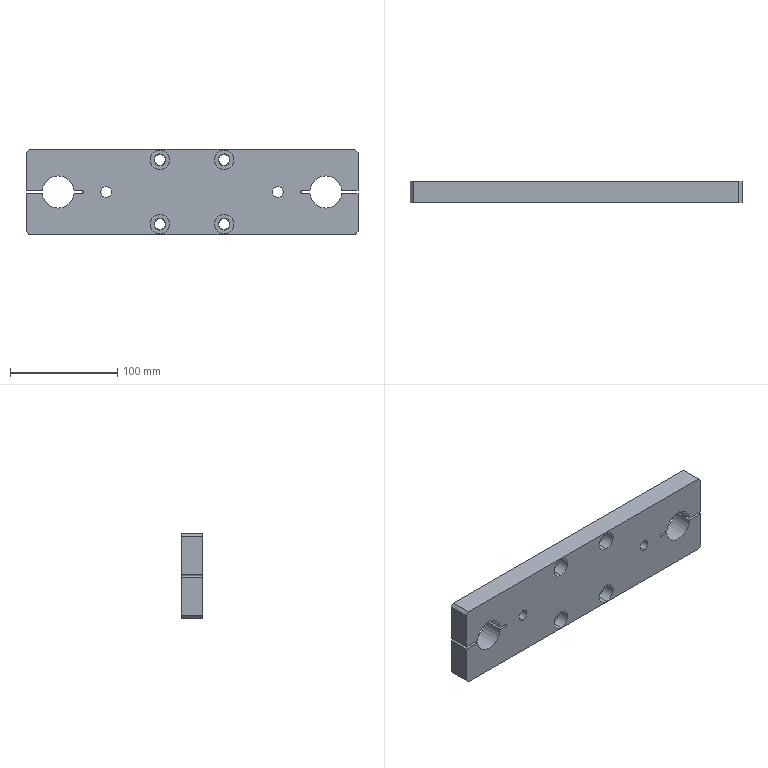Part | SolidWorks | features HoleWzd 4, ICE 2, Chamfer 1, Extrusion 1 | 1 solid | 78 faces | box 310 x 20 x 80 mm | volume 438735 mm3 | cylinder 40 | plane 26 | cone 12 | commonest cylinder face diameters 11 x8 18 x8 30 x6 6.8 x4 9 x4 10.2 x4